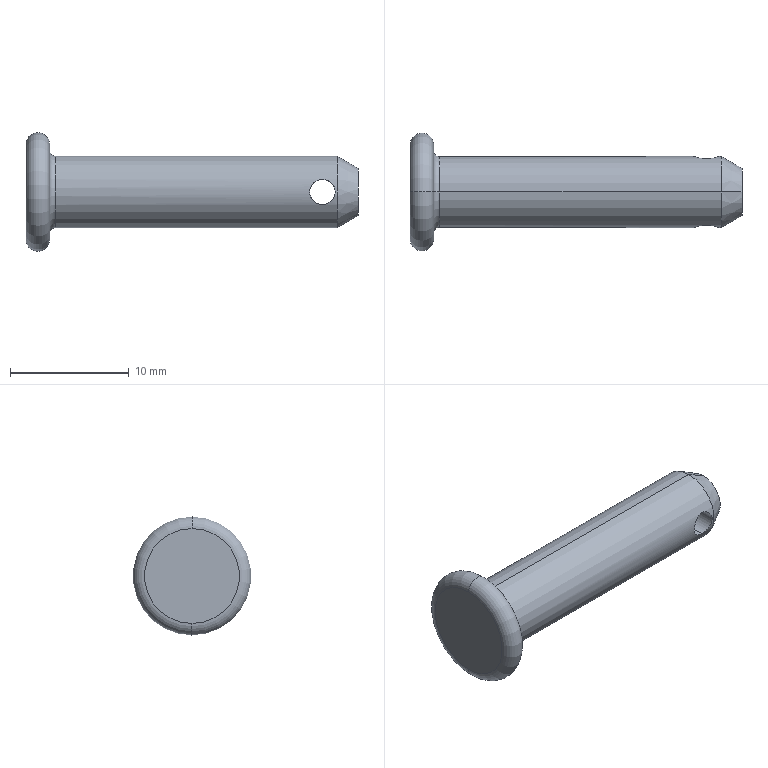Part | SolidWorks | features Chamfer 1, Cut 1, Fillet 1, Revolution 1 | 1 solid | 13 faces | box 28 x 10 x 10 mm | volume 844.638 mm3 | cylinder 4 | torus 4 | plane 3 | cone 2 | commonest cylinder face diameters 2.14 x2 6 x2
STEP:
#1=CARTESIAN_POINT('',(25.,-2.803,-1.07));
#2=VERTEX_POINT('',#1);
#3=CARTESIAN_POINT('',(25.,-2.803,1.07));
#4=VERTEX_POINT('',#3);
#5=CARTESIAN_POINT('',(25.,-2.803,-1.07));
#6=CARTESIAN_POINT('',(24.86,-2.803,-1.07));
#7=CARTESIAN_POINT('',(24.718,-2.814,-1.042));
#8=CARTESIAN_POINT('',(24.46,-2.851,-0.934));
#9=CARTESIAN_POINT('',(24.342,-2.877,-0.8554));
#10=CARTESIAN_POINT('',(24.144,-2.929,-0.6576));
#11=CARTESIAN_POINT('',(24.066,-2.954,-0.5409));
#12=CARTESIAN_POINT('',(23.958,-2.99,-0.2812));
#13=CARTESIAN_POINT('',(23.93,-3.,-0.1407));
#14=CARTESIAN_POINT('',(23.93,-3.,0.1413));
#15=CARTESIAN_POINT('',(23.959,-2.989,0.2829));
#16=CARTESIAN_POINT('',(24.066,-2.954,0.5407));
#17=CARTESIAN_POINT('',(24.146,-2.929,0.6589));
#18=CARTESIAN_POINT('',(24.342,-2.877,0.855));
#19=CARTESIAN_POINT('',(24.459,-2.852,0.9338));
#20=CARTESIAN_POINT('',(24.718,-2.814,1.042));
#21=CARTESIAN_POINT('',(24.857,-2.803,1.07));
#22=CARTESIAN_POINT('',(25.,-2.803,1.07));
#23=B_SPLINE_CURVE_WITH_KNOTS('',3,(#5,#6,#7,#8,#9,#10,#11,#12,#13,#14,#15,#16,#17,#18,#19,#20,#21,#22),.UNSPECIFIED.,.F.,.F.,(4,2,2,2,2,2,2,2,4),(0.003373,0.003795,0.004216,0.004638,0.005059,0.005481,0.005903,0.006324,0.006746),.UNSPECIFIED.);
#24=EDGE_CURVE('',#2,#4,#23,.T.);
#25=ORIENTED_EDGE('',*,*,#24,.F.);
#26=CARTESIAN_POINT('',(25.,2.803,-1.07));
#27=VERTEX_POINT('',#26);
#28=CARTESIAN_POINT('',(25.,-500.,-1.07));
#29=DIRECTION('',(0.,1.,0.));
#30=VECTOR('',#29,1000.);
#31=LINE('',#28,#30);
#32=EDGE_CURVE('',#2,#27,#31,.T.);
#33=ORIENTED_EDGE('',*,*,#32,.T.);
#34=CARTESIAN_POINT('',(25.,2.803,1.07));
#35=VERTEX_POINT('',#34);
#36=CARTESIAN_POINT('',(25.,2.803,1.07));
#37=CARTESIAN_POINT('',(24.857,2.803,1.07));
#38=CARTESIAN_POINT('',(24.717,2.814,1.041));
#39=CARTESIAN_POINT('',(24.459,2.852,0.9337));
#40=CARTESIAN_POINT('',(24.341,2.878,0.8543));
#41=CARTESIAN_POINT('',(24.145,2.929,0.6586));
#42=CARTESIAN_POINT('',(24.066,2.954,0.5402));
#43=CARTESIAN_POINT('',(23.959,2.989,0.2831));
#44=CARTESIAN_POINT('',(23.93,3.,0.1415));
#45=CARTESIAN_POINT('',(23.93,3.,-0.1404));
#46=CARTESIAN_POINT('',(23.958,2.99,-0.2811));
#47=CARTESIAN_POINT('',(24.067,2.954,-0.5419));
#48=CARTESIAN_POINT('',(24.146,2.928,-0.6589));
#49=CARTESIAN_POINT('',(24.342,2.877,-0.8554));
#50=CARTESIAN_POINT('',(24.46,2.851,-0.9344));
#51=CARTESIAN_POINT('',(24.718,2.814,-1.041));
#52=CARTESIAN_POINT('',(24.86,2.803,-1.07));
#53=CARTESIAN_POINT('',(25.,2.803,-1.07));
#54=B_SPLINE_CURVE_WITH_KNOTS('',3,(#36,#37,#38,#39,#40,#41,#42,#43,#44,#45,#46,#47,#48,#49,#50,#51,#52,#53),.UNSPECIFIED.,.F.,.F.,(4,2,2,2,2,2,2,2,4),(0.,0.0004217,0.0008433,0.001265,0.001687,0.002108,0.00253,0.002952,0.003373),.UNSPECIFIED.);
#55=EDGE_CURVE('',#35,#27,#54,.T.);
#56=ORIENTED_EDGE('',*,*,#55,.F.);
#57=CARTESIAN_POINT('',(25.,-500.,1.07));
#58=DIRECTION('',(0.,1.,0.));
#59=VECTOR('',#58,1000.);
#60=LINE('',#57,#59);
#61=EDGE_CURVE('',#4,#35,#60,.T.);
#62=ORIENTED_EDGE('',*,*,#61,.F.);
#63=EDGE_LOOP('',(#25,#33,#56,#62));
#64=FACE_OUTER_BOUND('',#63,.T.);
#65=CARTESIAN_POINT('',(25.,-500.,0.));
#66=DIRECTION('',(0.,1.,0.));
#67=DIRECTION('',(0.,0.,1.));
#68=AXIS2_PLACEMENT_3D('',#65,#66,#67);
#69=CYLINDRICAL_SURFACE('',#68,1.07);
#70=ADVANCED_FACE('',(#64),#69,.F.);
#71=CARTESIAN_POINT('',(28.,0.,-2.));
#72=VERTEX_POINT('',#71);
#73=CARTESIAN_POINT('',(28.,0.,2.));
#74=VERTEX_POINT('',#73);
#75=CARTESIAN_POINT('',(28.,0.,0.));
#76=DIRECTION('',(1.,0.,0.));
#77=DIRECTION('',(0.,0.,1.));
#78=AXIS2_PLACEMENT_3D('',#75,#76,#77);
#79=CIRCLE('',#78,2.);
#80=EDGE_CURVE('',#72,#74,#79,.T.);
#81=ORIENTED_EDGE('',*,*,#80,.F.);
#82=CARTESIAN_POINT('',(26.268,0.,-3.));
#83=VERTEX_POINT('',#82);
#84=CARTESIAN_POINT('',(26.268,0.,-3.));
#85=DIRECTION('',(-0.866,0.,-0.5));
#86=VECTOR('',#85,1000.);
#87=LINE('',#84,#86);
#88=EDGE_CURVE('',#72,#83,#87,.T.);
#89=ORIENTED_EDGE('',*,*,#88,.T.);
#90=CARTESIAN_POINT('',(26.268,0.,3.));
#91=VERTEX_POINT('',#90);
#92=CARTESIAN_POINT('',(26.268,0.,0.));
#93=DIRECTION('',(-1.,0.,0.));
#94=DIRECTION('',(0.,0.,1.));
#95=AXIS2_PLACEMENT_3D('',#92,#93,#94);
#96=CIRCLE('',#95,3.);
#97=EDGE_CURVE('',#91,#83,#96,.T.);
#98=ORIENTED_EDGE('',*,*,#97,.F.);
#99=CARTESIAN_POINT('',(26.268,0.,3.));
#100=DIRECTION('',(-0.866,0.,0.5));
#101=VECTOR('',#100,1000.);
#102=LINE('',#99,#101);
#103=EDGE_CURVE('',#74,#91,#102,.T.);
#104=ORIENTED_EDGE('',*,*,#103,.F.);
#105=EDGE_LOOP('',(#81,#89,#98,#104));
#106=FACE_OUTER_BOUND('',#105,.T.);
#107=CARTESIAN_POINT('',(26.268,0.,0.));
#108=DIRECTION('',(-1.,0.,0.));
#109=DIRECTION('',(0.,0.,1.));
#110=AXIS2_PLACEMENT_3D('',#107,#108,#109);
#111=CONICAL_SURFACE('',#110,3.,0.5236);
#112=ADVANCED_FACE('',(#106),#111,.T.);
#113=CARTESIAN_POINT('',(2.,0.,-3.5));
#114=VERTEX_POINT('',#113);
#115=CARTESIAN_POINT('',(2.,0.,3.5));
#116=VERTEX_POINT('',#115);
#117=CARTESIAN_POINT('',(2.,0.,0.));
#118=DIRECTION('',(-1.,0.,0.));
#119=DIRECTION('',(0.,0.,1.));
#120=AXIS2_PLACEMENT_3D('',#117,#118,#119);
#121=CIRCLE('',#120,3.5);
#122=EDGE_CURVE('',#114,#116,#121,.T.);
#123=ORIENTED_EDGE('',*,*,#122,.F.);
#124=CARTESIAN_POINT('',(2.5,0.,-3.));
#125=VERTEX_POINT('',#124);
#126=CARTESIAN_POINT('',(2.5,0.,-3.5));
#127=DIRECTION('',(0.,1.,0.));
#128=DIRECTION('',(0.,0.,1.));
#129=AXIS2_PLACEMENT_3D('',#126,#127,#128);
#130=CIRCLE('',#129,0.5);
#131=EDGE_CURVE('',#114,#125,#130,.T.);
#132=ORIENTED_EDGE('',*,*,#131,.T.);
#133=CARTESIAN_POINT('',(2.5,0.,3.));
#134=VERTEX_POINT('',#133);
#135=CARTESIAN_POINT('',(2.5,0.,0.));
#136=DIRECTION('',(1.,0.,0.));
#137=DIRECTION('',(0.,0.,1.));
#138=AXIS2_PLACEMENT_3D('',#135,#136,#137);
#139=CIRCLE('',#138,3.);
#140=EDGE_CURVE('',#134,#125,#139,.T.);
#141=ORIENTED_EDGE('',*,*,#140,.F.);
#142=CARTESIAN_POINT('',(2.5,0.,3.5));
#143=DIRECTION('',(0.,-1.,0.));
#144=DIRECTION('',(0.,0.,-1.));
#145=AXIS2_PLACEMENT_3D('',#142,#143,#144);
#146=CIRCLE('',#145,0.5);
#147=EDGE_CURVE('',#116,#134,#146,.T.);
#148=ORIENTED_EDGE('',*,*,#147,.F.);
#149=EDGE_LOOP('',(#123,#132,#141,#148));
#150=FACE_OUTER_BOUND('',#149,.T.);
#151=CARTESIAN_POINT('',(2.5,0.,0.));
#152=DIRECTION('',(-1.,0.,0.));
#153=DIRECTION('',(0.,0.,1.));
#154=AXIS2_PLACEMENT_3D('',#151,#152,#153);
#155=TOROIDAL_SURFACE('',#154,3.5,0.5);
#156=ADVANCED_FACE('',(#150),#155,.F.);
#157=ORIENTED_EDGE('',*,*,#55,.T.);
#158=CARTESIAN_POINT('',(25.,2.803,-1.07));
#159=CARTESIAN_POINT('',(25.14,2.803,-1.07));
#160=CARTESIAN_POINT('',(25.282,2.814,-1.042));
#161=CARTESIAN_POINT('',(25.54,2.851,-0.934));
#162=CARTESIAN_POINT('',(25.658,2.877,-0.8554));
#163=CARTESIAN_POINT('',(25.856,2.929,-0.6576));
#164=CARTESIAN_POINT('',(25.934,2.954,-0.5409));
#165=CARTESIAN_POINT('',(26.042,2.99,-0.2812));
#166=CARTESIAN_POINT('',(26.07,3.,-0.1407));
#167=CARTESIAN_POINT('',(26.07,3.,0.1413));
#168=CARTESIAN_POINT('',(26.041,2.989,0.2829));
#169=CARTESIAN_POINT('',(25.934,2.954,0.5407));
#170=CARTESIAN_POINT('',(25.854,2.929,0.6589));
#171=CARTESIAN_POINT('',(25.658,2.877,0.855));
#172=CARTESIAN_POINT('',(25.541,2.852,0.9338));
#173=CARTESIAN_POINT('',(25.282,2.814,1.042));
#174=CARTESIAN_POINT('',(25.143,2.803,1.07));
#175=CARTESIAN_POINT('',(25.,2.803,1.07));
#176=B_SPLINE_CURVE_WITH_KNOTS('',3,(#158,#159,#160,#161,#162,#163,#164,#165,#166,#167,#168,#169,#170,#171,#172,#173,#174,#175),.UNSPECIFIED.,.F.,.F.,(4,2,2,2,2,2,2,2,4),(0.003373,0.003795,0.004216,0.004638,0.005059,0.005481,0.005903,0.006324,0.006746),.UNSPECIFIED.);
#177=EDGE_CURVE('',#27,#35,#176,.T.);
#178=ORIENTED_EDGE('',*,*,#177,.T.);
#179=EDGE_LOOP('',(#157,#178));
#180=FACE_BOUND('',#179,.T.);
#181=ORIENTED_EDGE('',*,*,#97,.T.);
#182=CARTESIAN_POINT('',(0.,0.,-3.));
#183=DIRECTION('',(-1.,0.,0.));
#184=VECTOR('',#183,1000.);
#185=LINE('',#182,#184);
#186=EDGE_CURVE('',#83,#125,#185,.T.);
#187=ORIENTED_EDGE('',*,*,#186,.T.);
#188=CARTESIAN_POINT('',(2.5,0.,0.));
#189=DIRECTION('',(1.,0.,0.));
#190=DIRECTION('',(0.,0.,1.));
#191=AXIS2_PLACEMENT_3D('',#188,#189,#190);
#192=CIRCLE('',#191,3.);
#193=EDGE_CURVE('',#125,#134,#192,.T.);
#194=ORIENTED_EDGE('',*,*,#193,.T.);
#195=CARTESIAN_POINT('',(0.,0.,3.));
#196=DIRECTION('',(-1.,0.,0.));
#197=VECTOR('',#196,1000.);
#198=LINE('',#195,#197);
#199=EDGE_CURVE('',#91,#134,#198,.T.);
#200=ORIENTED_EDGE('',*,*,#199,.F.);
#201=EDGE_LOOP('',(#181,#187,#194,#200));
#202=FACE_OUTER_BOUND('',#201,.T.);
#203=CARTESIAN_POINT('',(0.,0.,0.));
#204=DIRECTION('',(-1.,0.,0.));
#205=DIRECTION('',(0.,0.,1.));
#206=AXIS2_PLACEMENT_3D('',#203,#204,#205);
#207=CYLINDRICAL_SURFACE('',#206,3.);
#208=ADVANCED_FACE('',(#180,#202),#207,.T.);
#209=CARTESIAN_POINT('',(2.,0.,4.));
#210=VERTEX_POINT('',#209);
#211=CARTESIAN_POINT('',(2.,0.,-4.));
#212=VERTEX_POINT('',#211);
#213=CARTESIAN_POINT('',(2.,0.,0.));
#214=DIRECTION('',(-1.,0.,0.));
#215=DIRECTION('',(0.,0.,1.));
#216=AXIS2_PLACEMENT_3D('',#213,#214,#215);
#217=CIRCLE('',#216,4.);
#218=EDGE_CURVE('',#210,#212,#217,.T.);
#219=ORIENTED_EDGE('',*,*,#218,.T.);
#220=CARTESIAN_POINT('',(0.,0.,-4.));
#221=VERTEX_POINT('',#220);
#222=CARTESIAN_POINT('',(1.,0.,-4.));
#223=DIRECTION('',(0.,1.,0.));
#224=DIRECTION('',(0.,0.,1.));
#225=AXIS2_PLACEMENT_3D('',#222,#223,#224);
#226=CIRCLE('',#225,1.);
#227=EDGE_CURVE('',#212,#221,#226,.T.);
#228=ORIENTED_EDGE('',*,*,#227,.T.);
#229=CARTESIAN_POINT('',(0.,0.,4.));
#230=VERTEX_POINT('',#229);
#231=CARTESIAN_POINT('',(0.,0.,0.));
#232=DIRECTION('',(-1.,0.,0.));
#233=DIRECTION('',(0.,0.,1.));
#234=AXIS2_PLACEMENT_3D('',#231,#232,#233);
#235=CIRCLE('',#234,4.);
#236=EDGE_CURVE('',#230,#221,#235,.T.);
#237=ORIENTED_EDGE('',*,*,#236,.F.);
#238=CARTESIAN_POINT('',(1.,0.,4.));
#239=DIRECTION('',(0.,-1.,0.));
#240=DIRECTION('',(0.,0.,-1.));
#241=AXIS2_PLACEMENT_3D('',#238,#239,#240);
#242=CIRCLE('',#241,1.);
#243=EDGE_CURVE('',#210,#230,#242,.T.);
#244=ORIENTED_EDGE('',*,*,#243,.F.);
#245=EDGE_LOOP('',(#219,#228,#237,#244));
#246=FACE_OUTER_BOUND('',#245,.T.);
#247=CARTESIAN_POINT('',(1.,0.,0.));
#248=DIRECTION('',(-1.,0.,0.));
#249=DIRECTION('',(0.,0.,1.));
#250=AXIS2_PLACEMENT_3D('',#247,#248,#249);
#251=TOROIDAL_SURFACE('',#250,4.,1.);
#252=ADVANCED_FACE('',(#246),#251,.T.);
#253=ORIENTED_EDGE('',*,*,#236,.T.);
#254=CARTESIAN_POINT('',(0.,0.,0.));
#255=DIRECTION('',(-1.,0.,0.));
#256=DIRECTION('',(0.,0.,1.));
#257=AXIS2_PLACEMENT_3D('',#254,#255,#256);
#258=CIRCLE('',#257,4.);
#259=EDGE_CURVE('',#221,#230,#258,.T.);
#260=ORIENTED_EDGE('',*,*,#259,.T.);
#261=EDGE_LOOP('',(#253,#260));
#262=FACE_OUTER_BOUND('',#261,.T.);
#263=CARTESIAN_POINT('',(0.,0.,0.));
#264=DIRECTION('',(1.,0.,0.));
#265=DIRECTION('',(0.,0.,-1.));
#266=AXIS2_PLACEMENT_3D('',#263,#264,#265);
#267=PLANE('',#266);
#268=ADVANCED_FACE('',(#262),#267,.F.);
#269=ORIENTED_EDGE('',*,*,#227,.F.);
#270=CARTESIAN_POINT('',(2.,0.,0.));
#271=DIRECTION('',(-1.,0.,0.));
#272=DIRECTION('',(0.,0.,1.));
#273=AXIS2_PLACEMENT_3D('',#270,#271,#272);
#274=CIRCLE('',#273,4.);
#275=EDGE_CURVE('',#212,#210,#274,.T.);
#276=ORIENTED_EDGE('',*,*,#275,.T.);
#277=ORIENTED_EDGE('',*,*,#243,.T.);
#278=ORIENTED_EDGE('',*,*,#259,.F.);
#279=EDGE_LOOP('',(#269,#276,#277,#278));
#280=FACE_OUTER_BOUND('',#279,.T.);
#281=CARTESIAN_POINT('',(1.,0.,0.));
#282=DIRECTION('',(-1.,0.,0.));
#283=DIRECTION('',(0.,0.,1.));
#284=AXIS2_PLACEMENT_3D('',#281,#282,#283);
#285=TOROIDAL_SURFACE('',#284,4.,1.);
#286=ADVANCED_FACE('',(#280),#285,.T.);
#287=CARTESIAN_POINT('',(2.,0.,0.));
#288=DIRECTION('',(-1.,0.,0.));
#289=DIRECTION('',(0.,0.,1.));
#290=AXIS2_PLACEMENT_3D('',#287,#288,#289);
#291=CIRCLE('',#290,3.5);
#292=EDGE_CURVE('',#116,#114,#291,.T.);
#293=ORIENTED_EDGE('',*,*,#292,.T.);
#294=ORIENTED_EDGE('',*,*,#122,.T.);
#295=EDGE_LOOP('',(#293,#294));
#296=FACE_BOUND('',#295,.T.);
#297=ORIENTED_EDGE('',*,*,#218,.F.);
#298=ORIENTED_EDGE('',*,*,#275,.F.);
#299=EDGE_LOOP('',(#297,#298));
#300=FACE_OUTER_BOUND('',#299,.T.);
#301=CARTESIAN_POINT('',(2.,4.,0.));
#302=DIRECTION('',(-1.,0.,0.));
#303=DIRECTION('',(0.,0.,1.));
#304=AXIS2_PLACEMENT_3D('',#301,#302,#303);
#305=PLANE('',#304);
#306=ADVANCED_FACE('',(#296,#300),#305,.F.);
#307=ORIENTED_EDGE('',*,*,#186,.F.);
#308=CARTESIAN_POINT('',(26.268,0.,0.));
#309=DIRECTION('',(-1.,0.,0.));
#310=DIRECTION('',(0.,0.,1.));
#311=AXIS2_PLACEMENT_3D('',#308,#309,#310);
#312=CIRCLE('',#311,3.);
#313=EDGE_CURVE('',#83,#91,#312,.T.);
#314=ORIENTED_EDGE('',*,*,#313,.T.);
#315=ORIENTED_EDGE('',*,*,#199,.T.);
#316=ORIENTED_EDGE('',*,*,#140,.T.);
#317=EDGE_LOOP('',(#307,#314,#315,#316));
#318=FACE_OUTER_BOUND('',#317,.T.);
#319=CARTESIAN_POINT('',(25.,-2.803,1.07));
#320=CARTESIAN_POINT('',(25.143,-2.803,1.07));
#321=CARTESIAN_POINT('',(25.283,-2.814,1.041));
#322=CARTESIAN_POINT('',(25.541,-2.852,0.9337));
#323=CARTESIAN_POINT('',(25.659,-2.878,0.8543));
#324=CARTESIAN_POINT('',(25.855,-2.929,0.6586));
#325=CARTESIAN_POINT('',(25.934,-2.954,0.5402));
#326=CARTESIAN_POINT('',(26.041,-2.989,0.2831));
#327=CARTESIAN_POINT('',(26.07,-3.,0.1415));
#328=CARTESIAN_POINT('',(26.07,-3.,-0.1404));
#329=CARTESIAN_POINT('',(26.042,-2.99,-0.2811));
#330=CARTESIAN_POINT('',(25.933,-2.954,-0.5419));
#331=CARTESIAN_POINT('',(25.854,-2.928,-0.6589));
#332=CARTESIAN_POINT('',(25.658,-2.877,-0.8554));
#333=CARTESIAN_POINT('',(25.54,-2.851,-0.9344));
#334=CARTESIAN_POINT('',(25.282,-2.814,-1.041));
#335=CARTESIAN_POINT('',(25.14,-2.803,-1.07));
#336=CARTESIAN_POINT('',(25.,-2.803,-1.07));
#337=B_SPLINE_CURVE_WITH_KNOTS('',3,(#319,#320,#321,#322,#323,#324,#325,#326,#327,#328,#329,#330,#331,#332,#333,#334,#335,#336),.UNSPECIFIED.,.F.,.F.,(4,2,2,2,2,2,2,2,4),(0.,0.0004217,0.0008433,0.001265,0.001687,0.002108,0.00253,0.002952,0.003373),.UNSPECIFIED.);
#338=EDGE_CURVE('',#4,#2,#337,.T.);
#339=ORIENTED_EDGE('',*,*,#338,.T.);
#340=ORIENTED_EDGE('',*,*,#24,.T.);
#341=EDGE_LOOP('',(#339,#340));
#342=FACE_BOUND('',#341,.T.);
#343=CARTESIAN_POINT('',(0.,0.,0.));
#344=DIRECTION('',(-1.,0.,0.));
#345=DIRECTION('',(0.,0.,1.));
#346=AXIS2_PLACEMENT_3D('',#343,#344,#345);
#347=CYLINDRICAL_SURFACE('',#346,3.);
#348=ADVANCED_FACE('',(#318,#342),#347,.T.);
#349=CARTESIAN_POINT('',(28.,0.,0.));
#350=DIRECTION('',(1.,0.,0.));
#351=DIRECTION('',(0.,0.,1.));
#352=AXIS2_PLACEMENT_3D('',#349,#350,#351);
#353=CIRCLE('',#352,2.);
#354=EDGE_CURVE('',#74,#72,#353,.T.);
#355=ORIENTED_EDGE('',*,*,#354,.T.);
#356=ORIENTED_EDGE('',*,*,#80,.T.);
#357=EDGE_LOOP('',(#355,#356));
#358=FACE_OUTER_BOUND('',#357,.T.);
#359=CARTESIAN_POINT('',(28.,3.,0.));
#360=DIRECTION('',(-1.,0.,0.));
#361=DIRECTION('',(0.,0.,1.));
#362=AXIS2_PLACEMENT_3D('',#359,#360,#361);
#363=PLANE('',#362);
#364=ADVANCED_FACE('',(#358),#363,.F.);
#365=ORIENTED_EDGE('',*,*,#131,.F.);
#366=ORIENTED_EDGE('',*,*,#292,.F.);
#367=ORIENTED_EDGE('',*,*,#147,.T.);
#368=ORIENTED_EDGE('',*,*,#193,.F.);
#369=EDGE_LOOP('',(#365,#366,#367,#368));
#370=FACE_OUTER_BOUND('',#369,.T.);
#371=CARTESIAN_POINT('',(2.5,0.,0.));
#372=DIRECTION('',(-1.,0.,0.));
#373=DIRECTION('',(0.,0.,1.));
#374=AXIS2_PLACEMENT_3D('',#371,#372,#373);
#375=TOROIDAL_SURFACE('',#374,3.5,0.5);
#376=ADVANCED_FACE('',(#370),#375,.F.);
#377=ORIENTED_EDGE('',*,*,#88,.F.);
#378=ORIENTED_EDGE('',*,*,#354,.F.);
#379=ORIENTED_EDGE('',*,*,#103,.T.);
#380=ORIENTED_EDGE('',*,*,#313,.F.);
#381=EDGE_LOOP('',(#377,#378,#379,#380));
#382=FACE_OUTER_BOUND('',#381,.T.);
#383=CARTESIAN_POINT('',(26.268,0.,0.));
#384=DIRECTION('',(-1.,0.,0.));
#385=DIRECTION('',(0.,0.,1.));
#386=AXIS2_PLACEMENT_3D('',#383,#384,#385);
#387=CONICAL_SURFACE('',#386,3.,0.5236);
#388=ADVANCED_FACE('',(#382),#387,.T.);
#389=ORIENTED_EDGE('',*,*,#32,.F.);
#390=ORIENTED_EDGE('',*,*,#338,.F.);
#391=ORIENTED_EDGE('',*,*,#61,.T.);
#392=ORIENTED_EDGE('',*,*,#177,.F.);
#393=EDGE_LOOP('',(#389,#390,#391,#392));
#394=FACE_OUTER_BOUND('',#393,.T.);
#395=CARTESIAN_POINT('',(25.,-500.,0.));
#396=DIRECTION('',(0.,1.,0.));
#397=DIRECTION('',(0.,0.,1.));
#398=AXIS2_PLACEMENT_3D('',#395,#396,#397);
#399=CYLINDRICAL_SURFACE('',#398,1.07);
#400=ADVANCED_FACE('',(#394),#399,.F.);
#401=CLOSED_SHELL('',(#70,#112,#156,#208,#252,#268,#286,#306,#348,#364,#376,#388,#400));
#402=MANIFOLD_SOLID_BREP('',#401);
#403=CARTESIAN_POINT('',(0.,0.,0.));
#404=DIRECTION('',(0.,0.,1.));
#405=DIRECTION('',(1.,0.,0.));
#406=AXIS2_PLACEMENT_3D('',#403,#404,#405);
#407=(LENGTH_UNIT()NAMED_UNIT(*)SI_UNIT(.MILLI.,.METRE.));
#408=UNCERTAINTY_MEASURE_WITH_UNIT(LENGTH_MEASURE(0.00001),#407,'','');
#409=(NAMED_UNIT(*)PLANE_ANGLE_UNIT()SI_UNIT($,.RADIAN.));
#410=(NAMED_UNIT(*)SI_UNIT($,.STERADIAN.)SOLID_ANGLE_UNIT());
#411=(GEOMETRIC_REPRESENTATION_CONTEXT(3)GLOBAL_UNCERTAINTY_ASSIGNED_CONTEXT((#408))GLOBAL_UNIT_ASSIGNED_CONTEXT((#407,#409,#410))REPRESENTATION_CONTEXT('',''));
#412=ADVANCED_BREP_SHAPE_REPRESENTATION('',(#402,#406),#411);